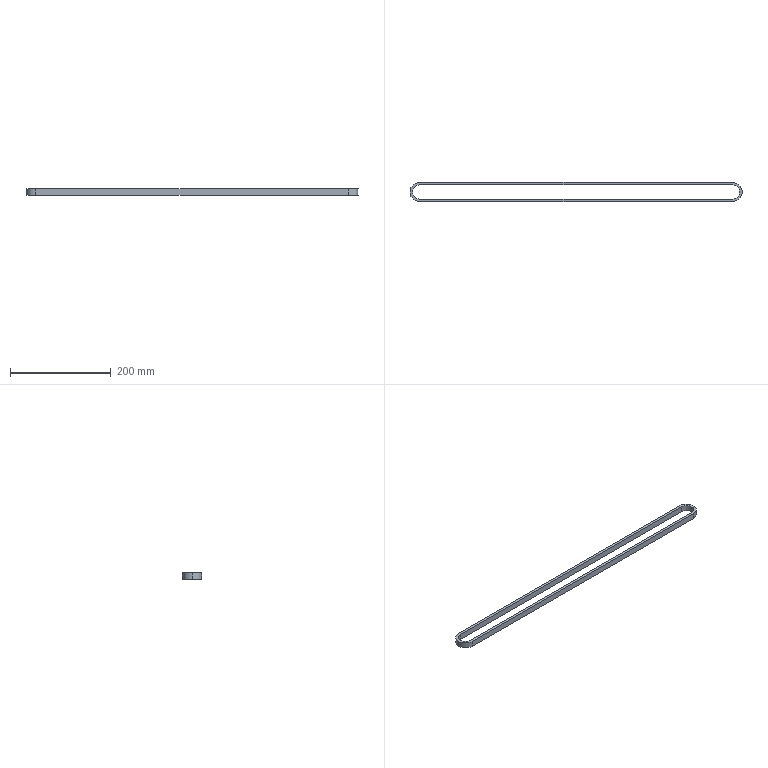Part | STEP file | 1/4in chain | 1 solid | 12 faces | box 658 x 38 x 12 mm | volume 80620 mm3 | cylinder 6 | plane 6 | commonest cylinder face diameters 28 x3 38 x3
STEP:
#1=CARTESIAN_POINT('',(0.,0.,0.));
#2=DIRECTION('',(0.,0.,1.));
#3=DIRECTION('',(1.,0.,0.));
#4=AXIS2_PLACEMENT_3D('',#1,#2,#3);
#5=CARTESIAN_POINT('',(-310.,14.,6.));
#6=VERTEX_POINT('',#5);
#7=CARTESIAN_POINT('',(-310.,14.,-6.));
#8=VERTEX_POINT('',#7);
#9=CARTESIAN_POINT('',(-310.,14.,6.));
#10=DIRECTION('',(0.,0.,-1.));
#11=VECTOR('',#10,1.);
#12=LINE('',#9,#11);
#13=CARTESIAN_POINT('',(-310.,0.,6.));
#14=DIRECTION('',(0.,0.,-1.));
#15=DIRECTION('',(-1.,0.,0.));
#16=AXIS2_PLACEMENT_3D('',#13,#14,#15);
#17=CYLINDRICAL_SURFACE('',#16,14.);
#18=CARTESIAN_POINT('',(1.571,0.));
#19=DIRECTION('',(0.,1.));
#20=VECTOR('',#19,1.);
#21=LINE('',#18,#20);
#22=(GEOMETRIC_REPRESENTATION_CONTEXT(2)PARAMETRIC_REPRESENTATION_CONTEXT()REPRESENTATION_CONTEXT('',''));
#23=DEFINITIONAL_REPRESENTATION('',(#21),#22);
#24=PCURVE('',#17,#23);
#25=CARTESIAN_POINT('',(-310.,14.,6.));
#26=DIRECTION('',(0.,-1.,0.));
#27=DIRECTION('',(1.,0.,0.));
#28=AXIS2_PLACEMENT_3D('',#25,#26,#27);
#29=PLANE('',#28);
#30=CARTESIAN_POINT('',(0.,0.));
#31=DIRECTION('',(0.,-1.));
#32=VECTOR('',#31,1.);
#33=LINE('',#30,#32);
#34=(GEOMETRIC_REPRESENTATION_CONTEXT(2)PARAMETRIC_REPRESENTATION_CONTEXT()REPRESENTATION_CONTEXT('',''));
#35=DEFINITIONAL_REPRESENTATION('',(#33),#34);
#36=PCURVE('',#29,#35);
#37=SURFACE_CURVE('',#12,(#24,#36),.PCURVE_S1.);
#38=EDGE_CURVE('',#6,#8,#37,.T.);
#39=ORIENTED_EDGE('',*,*,#38,.T.);
#40=CARTESIAN_POINT('',(-324.,0.,-6.));
#41=VERTEX_POINT('',#40);
#42=CARTESIAN_POINT('',(-310.,0.,-6.));
#43=DIRECTION('',(0.,0.,1.));
#44=DIRECTION('',(1.,0.,0.));
#45=AXIS2_PLACEMENT_3D('',#42,#43,#44);
#46=CIRCLE('',#45,14.);
#47=CARTESIAN_POINT('',(3.142,12.));
#48=DIRECTION('',(-1.,0.));
#49=VECTOR('',#48,1.);
#50=LINE('',#47,#49);
#51=(GEOMETRIC_REPRESENTATION_CONTEXT(2)PARAMETRIC_REPRESENTATION_CONTEXT()REPRESENTATION_CONTEXT('',''));
#52=DEFINITIONAL_REPRESENTATION('',(#50),#51);
#53=PCURVE('',#17,#52);
#54=CARTESIAN_POINT('',(-310.,0.,-6.));
#55=DIRECTION('',(0.,0.,1.));
#56=DIRECTION('',(1.,0.,0.));
#57=AXIS2_PLACEMENT_3D('',#54,#55,#56);
#58=PLANE('',#57);
#59=CARTESIAN_POINT('',(0.,0.));
#60=DIRECTION('',(1.,0.));
#61=AXIS2_PLACEMENT_2D('',#59,#60);
#62=CIRCLE('',#61,14.);
#63=(GEOMETRIC_REPRESENTATION_CONTEXT(2)PARAMETRIC_REPRESENTATION_CONTEXT()REPRESENTATION_CONTEXT('',''));
#64=DEFINITIONAL_REPRESENTATION('',(#62),#63);
#65=PCURVE('',#58,#64);
#66=SURFACE_CURVE('',#46,(#53,#65),.PCURVE_S1.);
#67=EDGE_CURVE('',#8,#41,#66,.T.);
#68=ORIENTED_EDGE('',*,*,#67,.T.);
#69=CARTESIAN_POINT('',(-324.,0.,6.));
#70=VERTEX_POINT('',#69);
#71=CARTESIAN_POINT('',(-324.,0.,6.));
#72=DIRECTION('',(0.,0.,-1.));
#73=VECTOR('',#72,1.);
#74=LINE('',#71,#73);
#75=CARTESIAN_POINT('',(0.,0.));
#76=DIRECTION('',(0.,1.));
#77=VECTOR('',#76,1.);
#78=LINE('',#75,#77);
#79=(GEOMETRIC_REPRESENTATION_CONTEXT(2)PARAMETRIC_REPRESENTATION_CONTEXT()REPRESENTATION_CONTEXT('',''));
#80=DEFINITIONAL_REPRESENTATION('',(#78),#79);
#81=PCURVE('',#17,#80);
#82=CARTESIAN_POINT('',(-310.,0.,6.));
#83=DIRECTION('',(0.,0.,-1.));
#84=DIRECTION('',(-1.,0.,0.));
#85=AXIS2_PLACEMENT_3D('',#82,#83,#84);
#86=CYLINDRICAL_SURFACE('',#85,14.);
#87=CARTESIAN_POINT('',(6.283,0.));
#88=DIRECTION('',(0.,1.));
#89=VECTOR('',#88,1.);
#90=LINE('',#87,#89);
#91=(GEOMETRIC_REPRESENTATION_CONTEXT(2)PARAMETRIC_REPRESENTATION_CONTEXT()REPRESENTATION_CONTEXT('',''));
#92=DEFINITIONAL_REPRESENTATION('',(#90),#91);
#93=PCURVE('',#86,#92);
#94=SURFACE_CURVE('',#74,(#81,#93),.PCURVE_S1.);
#95=EDGE_CURVE('',#70,#41,#94,.T.);
#96=ORIENTED_EDGE('',*,*,#95,.F.);
#97=CARTESIAN_POINT('',(-310.,0.,6.));
#98=DIRECTION('',(0.,0.,1.));
#99=DIRECTION('',(1.,0.,0.));
#100=AXIS2_PLACEMENT_3D('',#97,#98,#99);
#101=CIRCLE('',#100,14.);
#102=CARTESIAN_POINT('',(3.142,0.));
#103=DIRECTION('',(-1.,0.));
#104=VECTOR('',#103,1.);
#105=LINE('',#102,#104);
#106=(GEOMETRIC_REPRESENTATION_CONTEXT(2)PARAMETRIC_REPRESENTATION_CONTEXT()REPRESENTATION_CONTEXT('',''));
#107=DEFINITIONAL_REPRESENTATION('',(#105),#106);
#108=PCURVE('',#17,#107);
#109=CARTESIAN_POINT('',(-310.,0.,6.));
#110=DIRECTION('',(0.,0.,1.));
#111=DIRECTION('',(1.,0.,0.));
#112=AXIS2_PLACEMENT_3D('',#109,#110,#111);
#113=PLANE('',#112);
#114=CARTESIAN_POINT('',(0.,0.));
#115=DIRECTION('',(1.,0.));
#116=AXIS2_PLACEMENT_2D('',#114,#115);
#117=CIRCLE('',#116,14.);
#118=(GEOMETRIC_REPRESENTATION_CONTEXT(2)PARAMETRIC_REPRESENTATION_CONTEXT()REPRESENTATION_CONTEXT('',''));
#119=DEFINITIONAL_REPRESENTATION('',(#117),#118);
#120=PCURVE('',#113,#119);
#121=SURFACE_CURVE('',#101,(#108,#120),.PCURVE_S1.);
#122=EDGE_CURVE('',#6,#70,#121,.T.);
#123=ORIENTED_EDGE('',*,*,#122,.F.);
#124=EDGE_LOOP('',(#39,#68,#96,#123));
#125=FACE_BOUND('',#124,.F.);
#126=ADVANCED_FACE('',(#125),#17,.F.);
#127=CARTESIAN_POINT('',(-329.,0.,6.));
#128=VERTEX_POINT('',#127);
#129=CARTESIAN_POINT('',(-310.,-19.,6.));
#130=VERTEX_POINT('',#129);
#131=CARTESIAN_POINT('',(-310.,0.,6.));
#132=DIRECTION('',(0.,0.,1.));
#133=DIRECTION('',(1.,0.,0.));
#134=AXIS2_PLACEMENT_3D('',#131,#132,#133);
#135=CIRCLE('',#134,19.);
#136=CARTESIAN_POINT('',(-310.,0.,6.));
#137=DIRECTION('',(0.,0.,-1.));
#138=DIRECTION('',(-1.,0.,0.));
#139=AXIS2_PLACEMENT_3D('',#136,#137,#138);
#140=CYLINDRICAL_SURFACE('',#139,19.);
#141=CARTESIAN_POINT('',(9.425,0.));
#142=DIRECTION('',(-1.,0.));
#143=VECTOR('',#142,1.);
#144=LINE('',#141,#143);
#145=(GEOMETRIC_REPRESENTATION_CONTEXT(2)PARAMETRIC_REPRESENTATION_CONTEXT()REPRESENTATION_CONTEXT('',''));
#146=DEFINITIONAL_REPRESENTATION('',(#144),#145);
#147=PCURVE('',#140,#146);
#148=CARTESIAN_POINT('',(0.,0.));
#149=DIRECTION('',(1.,0.));
#150=AXIS2_PLACEMENT_2D('',#148,#149);
#151=CIRCLE('',#150,19.);
#152=(GEOMETRIC_REPRESENTATION_CONTEXT(2)PARAMETRIC_REPRESENTATION_CONTEXT()REPRESENTATION_CONTEXT('',''));
#153=DEFINITIONAL_REPRESENTATION('',(#151),#152);
#154=PCURVE('',#113,#153);
#155=SURFACE_CURVE('',#135,(#147,#154),.PCURVE_S1.);
#156=EDGE_CURVE('',#128,#130,#155,.T.);
#157=ORIENTED_EDGE('',*,*,#156,.F.);
#158=CARTESIAN_POINT('',(-329.,0.,-6.));
#159=VERTEX_POINT('',#158);
#160=CARTESIAN_POINT('',(-329.,0.,6.));
#161=DIRECTION('',(0.,0.,-1.));
#162=VECTOR('',#161,1.);
#163=LINE('',#160,#162);
#164=CARTESIAN_POINT('',(6.283,0.));
#165=DIRECTION('',(0.,1.));
#166=VECTOR('',#165,1.);
#167=LINE('',#164,#166);
#168=(GEOMETRIC_REPRESENTATION_CONTEXT(2)PARAMETRIC_REPRESENTATION_CONTEXT()REPRESENTATION_CONTEXT('',''));
#169=DEFINITIONAL_REPRESENTATION('',(#167),#168);
#170=PCURVE('',#140,#169);
#171=CARTESIAN_POINT('',(-310.,0.,6.));
#172=DIRECTION('',(0.,0.,-1.));
#173=DIRECTION('',(-1.,0.,0.));
#174=AXIS2_PLACEMENT_3D('',#171,#172,#173);
#175=CYLINDRICAL_SURFACE('',#174,19.);
#176=CARTESIAN_POINT('',(0.,0.));
#177=DIRECTION('',(0.,1.));
#178=VECTOR('',#177,1.);
#179=LINE('',#176,#178);
#180=(GEOMETRIC_REPRESENTATION_CONTEXT(2)PARAMETRIC_REPRESENTATION_CONTEXT()REPRESENTATION_CONTEXT('',''));
#181=DEFINITIONAL_REPRESENTATION('',(#179),#180);
#182=PCURVE('',#175,#181);
#183=SURFACE_CURVE('',#163,(#170,#182),.PCURVE_S1.);
#184=EDGE_CURVE('',#128,#159,#183,.T.);
#185=ORIENTED_EDGE('',*,*,#184,.T.);
#186=CARTESIAN_POINT('',(-310.,-19.,-6.));
#187=VERTEX_POINT('',#186);
#188=CARTESIAN_POINT('',(-310.,0.,-6.));
#189=DIRECTION('',(0.,0.,1.));
#190=DIRECTION('',(1.,0.,0.));
#191=AXIS2_PLACEMENT_3D('',#188,#189,#190);
#192=CIRCLE('',#191,19.);
#193=CARTESIAN_POINT('',(9.425,12.));
#194=DIRECTION('',(-1.,0.));
#195=VECTOR('',#194,1.);
#196=LINE('',#193,#195);
#197=(GEOMETRIC_REPRESENTATION_CONTEXT(2)PARAMETRIC_REPRESENTATION_CONTEXT()REPRESENTATION_CONTEXT('',''));
#198=DEFINITIONAL_REPRESENTATION('',(#196),#197);
#199=PCURVE('',#140,#198);
#200=CARTESIAN_POINT('',(0.,0.));
#201=DIRECTION('',(1.,0.));
#202=AXIS2_PLACEMENT_2D('',#200,#201);
#203=CIRCLE('',#202,19.);
#204=(GEOMETRIC_REPRESENTATION_CONTEXT(2)PARAMETRIC_REPRESENTATION_CONTEXT()REPRESENTATION_CONTEXT('',''));
#205=DEFINITIONAL_REPRESENTATION('',(#203),#204);
#206=PCURVE('',#58,#205);
#207=SURFACE_CURVE('',#192,(#199,#206),.PCURVE_S1.);
#208=EDGE_CURVE('',#159,#187,#207,.T.);
#209=ORIENTED_EDGE('',*,*,#208,.T.);
#210=CARTESIAN_POINT('',(-310.,-19.,6.));
#211=DIRECTION('',(0.,0.,-1.));
#212=VECTOR('',#211,1.);
#213=LINE('',#210,#212);
#214=CARTESIAN_POINT('',(4.712,0.));
#215=DIRECTION('',(0.,1.));
#216=VECTOR('',#215,1.);
#217=LINE('',#214,#216);
#218=(GEOMETRIC_REPRESENTATION_CONTEXT(2)PARAMETRIC_REPRESENTATION_CONTEXT()REPRESENTATION_CONTEXT('',''));
#219=DEFINITIONAL_REPRESENTATION('',(#217),#218);
#220=PCURVE('',#140,#219);
#221=CARTESIAN_POINT('',(-310.,-19.,6.));
#222=DIRECTION('',(0.,1.,0.));
#223=DIRECTION('',(-1.,0.,0.));
#224=AXIS2_PLACEMENT_3D('',#221,#222,#223);
#225=PLANE('',#224);
#226=CARTESIAN_POINT('',(0.,0.));
#227=DIRECTION('',(0.,-1.));
#228=VECTOR('',#227,1.);
#229=LINE('',#226,#228);
#230=(GEOMETRIC_REPRESENTATION_CONTEXT(2)PARAMETRIC_REPRESENTATION_CONTEXT()REPRESENTATION_CONTEXT('',''));
#231=DEFINITIONAL_REPRESENTATION('',(#229),#230);
#232=PCURVE('',#225,#231);
#233=SURFACE_CURVE('',#213,(#220,#232),.PCURVE_S1.);
#234=EDGE_CURVE('',#130,#187,#233,.T.);
#235=ORIENTED_EDGE('',*,*,#234,.F.);
#236=EDGE_LOOP('',(#157,#185,#209,#235));
#237=FACE_BOUND('',#236,.T.);
#238=ADVANCED_FACE('',(#237),#140,.T.);
#239=CARTESIAN_POINT('',(-310.,19.,6.));
#240=VERTEX_POINT('',#239);
#241=CARTESIAN_POINT('',(-310.,0.,6.));
#242=DIRECTION('',(0.,0.,1.));
#243=DIRECTION('',(1.,0.,0.));
#244=AXIS2_PLACEMENT_3D('',#241,#242,#243);
#245=CIRCLE('',#244,19.);
#246=CARTESIAN_POINT('',(0.,0.));
#247=DIRECTION('',(1.,0.));
#248=AXIS2_PLACEMENT_2D('',#246,#247);
#249=CIRCLE('',#248,19.);
#250=(GEOMETRIC_REPRESENTATION_CONTEXT(2)PARAMETRIC_REPRESENTATION_CONTEXT()REPRESENTATION_CONTEXT('',''));
#251=DEFINITIONAL_REPRESENTATION('',(#249),#250);
#252=PCURVE('',#113,#251);
#253=CARTESIAN_POINT('',(3.142,0.));
#254=DIRECTION('',(-1.,0.));
#255=VECTOR('',#254,1.);
#256=LINE('',#253,#255);
#257=(GEOMETRIC_REPRESENTATION_CONTEXT(2)PARAMETRIC_REPRESENTATION_CONTEXT()REPRESENTATION_CONTEXT('',''));
#258=DEFINITIONAL_REPRESENTATION('',(#256),#257);
#259=PCURVE('',#175,#258);
#260=SURFACE_CURVE('',#245,(#252,#259),.PCURVE_S1.);
#261=EDGE_CURVE('',#240,#128,#260,.T.);
#262=ORIENTED_EDGE('',*,*,#261,.T.);
#263=ORIENTED_EDGE('',*,*,#156,.T.);
#264=CARTESIAN_POINT('',(310.,-19.,6.));
#265=VERTEX_POINT('',#264);
#266=CARTESIAN_POINT('',(-310.,-19.,6.));
#267=DIRECTION('',(1.,0.,0.));
#268=VECTOR('',#267,1.);
#269=LINE('',#266,#268);
#270=CARTESIAN_POINT('',(0.,-19.));
#271=DIRECTION('',(1.,0.));
#272=VECTOR('',#271,1.);
#273=LINE('',#270,#272);
#274=(GEOMETRIC_REPRESENTATION_CONTEXT(2)PARAMETRIC_REPRESENTATION_CONTEXT()REPRESENTATION_CONTEXT('',''));
#275=DEFINITIONAL_REPRESENTATION('',(#273),#274);
#276=PCURVE('',#113,#275);
#277=CARTESIAN_POINT('',(0.,0.));
#278=DIRECTION('',(-1.,0.));
#279=VECTOR('',#278,1.);
#280=LINE('',#277,#279);
#281=(GEOMETRIC_REPRESENTATION_CONTEXT(2)PARAMETRIC_REPRESENTATION_CONTEXT()REPRESENTATION_CONTEXT('',''));
#282=DEFINITIONAL_REPRESENTATION('',(#280),#281);
#283=PCURVE('',#225,#282);
#284=SURFACE_CURVE('',#269,(#276,#283),.PCURVE_S1.);
#285=EDGE_CURVE('',#130,#265,#284,.T.);
#286=ORIENTED_EDGE('',*,*,#285,.T.);
#287=CARTESIAN_POINT('',(310.,19.,6.));
#288=VERTEX_POINT('',#287);
#289=CARTESIAN_POINT('',(310.,0.,6.));
#290=DIRECTION('',(0.,0.,1.));
#291=DIRECTION('',(-1.,0.,0.));
#292=AXIS2_PLACEMENT_3D('',#289,#290,#291);
#293=CIRCLE('',#292,19.);
#294=CARTESIAN_POINT('',(620.,0.));
#295=DIRECTION('',(-1.,0.));
#296=AXIS2_PLACEMENT_2D('',#294,#295);
#297=CIRCLE('',#296,19.);
#298=(GEOMETRIC_REPRESENTATION_CONTEXT(2)PARAMETRIC_REPRESENTATION_CONTEXT()REPRESENTATION_CONTEXT('',''));
#299=DEFINITIONAL_REPRESENTATION('',(#297),#298);
#300=PCURVE('',#113,#299);
#301=CARTESIAN_POINT('',(310.,0.,6.));
#302=DIRECTION('',(0.,0.,-1.));
#303=DIRECTION('',(-1.,0.,0.));
#304=AXIS2_PLACEMENT_3D('',#301,#302,#303);
#305=CYLINDRICAL_SURFACE('',#304,19.);
#306=CARTESIAN_POINT('',(6.283,0.));
#307=DIRECTION('',(-1.,0.));
#308=VECTOR('',#307,1.);
#309=LINE('',#306,#308);
#310=(GEOMETRIC_REPRESENTATION_CONTEXT(2)PARAMETRIC_REPRESENTATION_CONTEXT()REPRESENTATION_CONTEXT('',''));
#311=DEFINITIONAL_REPRESENTATION('',(#309),#310);
#312=PCURVE('',#305,#311);
#313=SURFACE_CURVE('',#293,(#300,#312),.PCURVE_S1.);
#314=EDGE_CURVE('',#265,#288,#313,.T.);
#315=ORIENTED_EDGE('',*,*,#314,.T.);
#316=CARTESIAN_POINT('',(-310.,19.,6.));
#317=DIRECTION('',(-1.,0.,0.));
#318=VECTOR('',#317,1.);
#319=LINE('',#316,#318);
#320=CARTESIAN_POINT('',(0.,19.));
#321=DIRECTION('',(-1.,0.));
#322=VECTOR('',#321,1.);
#323=LINE('',#320,#322);
#324=(GEOMETRIC_REPRESENTATION_CONTEXT(2)PARAMETRIC_REPRESENTATION_CONTEXT()REPRESENTATION_CONTEXT('',''));
#325=DEFINITIONAL_REPRESENTATION('',(#323),#324);
#326=PCURVE('',#113,#325);
#327=CARTESIAN_POINT('',(-310.,19.,6.));
#328=DIRECTION('',(0.,-1.,0.));
#329=DIRECTION('',(1.,0.,0.));
#330=AXIS2_PLACEMENT_3D('',#327,#328,#329);
#331=PLANE('',#330);
#332=CARTESIAN_POINT('',(0.,0.));
#333=DIRECTION('',(-1.,0.));
#334=VECTOR('',#333,1.);
#335=LINE('',#332,#334);
#336=(GEOMETRIC_REPRESENTATION_CONTEXT(2)PARAMETRIC_REPRESENTATION_CONTEXT()REPRESENTATION_CONTEXT('',''));
#337=DEFINITIONAL_REPRESENTATION('',(#335),#336);
#338=PCURVE('',#331,#337);
#339=SURFACE_CURVE('',#319,(#326,#338),.PCURVE_S1.);
#340=EDGE_CURVE('',#288,#240,#339,.T.);
#341=ORIENTED_EDGE('',*,*,#340,.T.);
#342=EDGE_LOOP('',(#262,#263,#286,#315,#341));
#343=FACE_BOUND('',#342,.T.);
#344=CARTESIAN_POINT('',(-310.,-14.,6.));
#345=VERTEX_POINT('',#344);
#346=CARTESIAN_POINT('',(310.,-14.,6.));
#347=VERTEX_POINT('',#346);
#348=CARTESIAN_POINT('',(-310.,-14.,6.));
#349=DIRECTION('',(1.,0.,0.));
#350=VECTOR('',#349,1.);
#351=LINE('',#348,#350);
#352=CARTESIAN_POINT('',(0.,-14.));
#353=DIRECTION('',(1.,0.));
#354=VECTOR('',#353,1.);
#355=LINE('',#352,#354);
#356=(GEOMETRIC_REPRESENTATION_CONTEXT(2)PARAMETRIC_REPRESENTATION_CONTEXT()REPRESENTATION_CONTEXT('',''));
#357=DEFINITIONAL_REPRESENTATION('',(#355),#356);
#358=PCURVE('',#113,#357);
#359=CARTESIAN_POINT('',(-310.,-14.,6.));
#360=DIRECTION('',(0.,1.,0.));
#361=DIRECTION('',(-1.,0.,0.));
#362=AXIS2_PLACEMENT_3D('',#359,#360,#361);
#363=PLANE('',#362);
#364=CARTESIAN_POINT('',(0.,0.));
#365=DIRECTION('',(-1.,0.));
#366=VECTOR('',#365,1.);
#367=LINE('',#364,#366);
#368=(GEOMETRIC_REPRESENTATION_CONTEXT(2)PARAMETRIC_REPRESENTATION_CONTEXT()REPRESENTATION_CONTEXT('',''));
#369=DEFINITIONAL_REPRESENTATION('',(#367),#368);
#370=PCURVE('',#363,#369);
#371=SURFACE_CURVE('',#351,(#358,#370),.PCURVE_S1.);
#372=EDGE_CURVE('',#345,#347,#371,.T.);
#373=ORIENTED_EDGE('',*,*,#372,.F.);
#374=CARTESIAN_POINT('',(-310.,0.,6.));
#375=DIRECTION('',(0.,0.,1.));
#376=DIRECTION('',(1.,0.,0.));
#377=AXIS2_PLACEMENT_3D('',#374,#375,#376);
#378=CIRCLE('',#377,14.);
#379=CARTESIAN_POINT('',(0.,0.));
#380=DIRECTION('',(1.,0.));
#381=AXIS2_PLACEMENT_2D('',#379,#380);
#382=CIRCLE('',#381,14.);
#383=(GEOMETRIC_REPRESENTATION_CONTEXT(2)PARAMETRIC_REPRESENTATION_CONTEXT()REPRESENTATION_CONTEXT('',''));
#384=DEFINITIONAL_REPRESENTATION('',(#382),#383);
#385=PCURVE('',#113,#384);
#386=CARTESIAN_POINT('',(9.425,0.));
#387=DIRECTION('',(-1.,0.));
#388=VECTOR('',#387,1.);
#389=LINE('',#386,#388);
#390=(GEOMETRIC_REPRESENTATION_CONTEXT(2)PARAMETRIC_REPRESENTATION_CONTEXT()REPRESENTATION_CONTEXT('',''));
#391=DEFINITIONAL_REPRESENTATION('',(#389),#390);
#392=PCURVE('',#86,#391);
#393=SURFACE_CURVE('',#378,(#385,#392),.PCURVE_S1.);
#394=EDGE_CURVE('',#70,#345,#393,.T.);
#395=ORIENTED_EDGE('',*,*,#394,.F.);
#396=ORIENTED_EDGE('',*,*,#122,.F.);
#397=CARTESIAN_POINT('',(310.,14.,6.));
#398=VERTEX_POINT('',#397);
#399=CARTESIAN_POINT('',(-310.,14.,6.));
#400=DIRECTION('',(-1.,0.,0.));
#401=VECTOR('',#400,1.);
#402=LINE('',#399,#401);
#403=CARTESIAN_POINT('',(0.,14.));
#404=DIRECTION('',(-1.,0.));
#405=VECTOR('',#404,1.);
#406=LINE('',#403,#405);
#407=(GEOMETRIC_REPRESENTATION_CONTEXT(2)PARAMETRIC_REPRESENTATION_CONTEXT()REPRESENTATION_CONTEXT('',''));
#408=DEFINITIONAL_REPRESENTATION('',(#406),#407);
#409=PCURVE('',#113,#408);
#410=CARTESIAN_POINT('',(0.,0.));
#411=DIRECTION('',(-1.,0.));
#412=VECTOR('',#411,1.);
#413=LINE('',#410,#412);
#414=(GEOMETRIC_REPRESENTATION_CONTEXT(2)PARAMETRIC_REPRESENTATION_CONTEXT()REPRESENTATION_CONTEXT('',''));
#415=DEFINITIONAL_REPRESENTATION('',(#413),#414);
#416=PCURVE('',#29,#415);
#417=SURFACE_CURVE('',#402,(#409,#416),.PCURVE_S1.);
#418=EDGE_CURVE('',#398,#6,#417,.T.);
#419=ORIENTED_EDGE('',*,*,#418,.F.);
#420=CARTESIAN_POINT('',(310.,0.,6.));
#421=DIRECTION('',(0.,0.,1.));
#422=DIRECTION('',(1.,0.,0.));
#423=AXIS2_PLACEMENT_3D('',#420,#421,#422);
#424=CIRCLE('',#423,14.);
#425=CARTESIAN_POINT('',(620.,0.));
#426=DIRECTION('',(1.,0.));
#427=AXIS2_PLACEMENT_2D('',#425,#426);
#428=CIRCLE('',#427,14.);
#429=(GEOMETRIC_REPRESENTATION_CONTEXT(2)PARAMETRIC_REPRESENTATION_CONTEXT()REPRESENTATION_CONTEXT('',''));
#430=DEFINITIONAL_REPRESENTATION('',(#428),#429);
#431=PCURVE('',#113,#430);
#432=CARTESIAN_POINT('',(310.,0.,6.));
#433=DIRECTION('',(0.,0.,-1.));
#434=DIRECTION('',(-1.,0.,0.));
#435=AXIS2_PLACEMENT_3D('',#432,#433,#434);
#436=CYLINDRICAL_SURFACE('',#435,14.);
#437=CARTESIAN_POINT('',(9.425,0.));
#438=DIRECTION('',(-1.,0.));
#439=VECTOR('',#438,1.);
#440=LINE('',#437,#439);
#441=(GEOMETRIC_REPRESENTATION_CONTEXT(2)PARAMETRIC_REPRESENTATION_CONTEXT()REPRESENTATION_CONTEXT('',''));
#442=DEFINITIONAL_REPRESENTATION('',(#440),#441);
#443=PCURVE('',#436,#442);
#444=SURFACE_CURVE('',#424,(#431,#443),.PCURVE_S1.);
#445=EDGE_CURVE('',#347,#398,#444,.T.);
#446=ORIENTED_EDGE('',*,*,#445,.F.);
#447=EDGE_LOOP('',(#373,#395,#396,#419,#446));
#448=FACE_BOUND('',#447,.T.);
#449=ADVANCED_FACE('',(#343,#448),#113,.T.);
#450=CARTESIAN_POINT('',(-310.,19.,-6.));
#451=VERTEX_POINT('',#450);
#452=CARTESIAN_POINT('',(-310.,0.,-6.));
#453=DIRECTION('',(0.,0.,1.));
#454=DIRECTION('',(1.,0.,0.));
#455=AXIS2_PLACEMENT_3D('',#452,#453,#454);
#456=CIRCLE('',#455,19.);
#457=CARTESIAN_POINT('',(0.,0.));
#458=DIRECTION('',(1.,0.));
#459=AXIS2_PLACEMENT_2D('',#457,#458);
#460=CIRCLE('',#459,19.);
#461=(GEOMETRIC_REPRESENTATION_CONTEXT(2)PARAMETRIC_REPRESENTATION_CONTEXT()REPRESENTATION_CONTEXT('',''));
#462=DEFINITIONAL_REPRESENTATION('',(#460),#461);
#463=PCURVE('',#58,#462);
#464=CARTESIAN_POINT('',(3.142,12.));
#465=DIRECTION('',(-1.,0.));
#466=VECTOR('',#465,1.);
#467=LINE('',#464,#466);
#468=(GEOMETRIC_REPRESENTATION_CONTEXT(2)PARAMETRIC_REPRESENTATION_CONTEXT()REPRESENTATION_CONTEXT('',''));
#469=DEFINITIONAL_REPRESENTATION('',(#467),#468);
#470=PCURVE('',#175,#469);
#471=SURFACE_CURVE('',#456,(#463,#470),.PCURVE_S1.);
#472=EDGE_CURVE('',#451,#159,#471,.T.);
#473=ORIENTED_EDGE('',*,*,#472,.F.);
#474=CARTESIAN_POINT('',(310.,19.,-6.));
#475=VERTEX_POINT('',#474);
#476=CARTESIAN_POINT('',(-310.,19.,-6.));
#477=DIRECTION('',(-1.,0.,0.));
#478=VECTOR('',#477,1.);
#479=LINE('',#476,#478);
#480=CARTESIAN_POINT('',(0.,19.));
#481=DIRECTION('',(-1.,0.));
#482=VECTOR('',#481,1.);
#483=LINE('',#480,#482);
#484=(GEOMETRIC_REPRESENTATION_CONTEXT(2)PARAMETRIC_REPRESENTATION_CONTEXT()REPRESENTATION_CONTEXT('',''));
#485=DEFINITIONAL_REPRESENTATION('',(#483),#484);
#486=PCURVE('',#58,#485);
#487=CARTESIAN_POINT('',(0.,-12.));
#488=DIRECTION('',(-1.,0.));
#489=VECTOR('',#488,1.);
#490=LINE('',#487,#489);
#491=(GEOMETRIC_REPRESENTATION_CONTEXT(2)PARAMETRIC_REPRESENTATION_CONTEXT()REPRESENTATION_CONTEXT('',''));
#492=DEFINITIONAL_REPRESENTATION('',(#490),#491);
#493=PCURVE('',#331,#492);
#494=SURFACE_CURVE('',#479,(#486,#493),.PCURVE_S1.);
#495=EDGE_CURVE('',#475,#451,#494,.T.);
#496=ORIENTED_EDGE('',*,*,#495,.F.);
#497=CARTESIAN_POINT('',(310.,-19.,-6.));
#498=VERTEX_POINT('',#497);
#499=CARTESIAN_POINT('',(310.,0.,-6.));
#500=DIRECTION('',(0.,0.,1.));
#501=DIRECTION('',(-1.,0.,0.));
#502=AXIS2_PLACEMENT_3D('',#499,#500,#501);
#503=CIRCLE('',#502,19.);
#504=CARTESIAN_POINT('',(620.,0.));
#505=DIRECTION('',(-1.,0.));
#506=AXIS2_PLACEMENT_2D('',#504,#505);
#507=CIRCLE('',#506,19.);
#508=(GEOMETRIC_REPRESENTATION_CONTEXT(2)PARAMETRIC_REPRESENTATION_CONTEXT()REPRESENTATION_CONTEXT('',''));
#509=DEFINITIONAL_REPRESENTATION('',(#507),#508);
#510=PCURVE('',#58,#509);
#511=CARTESIAN_POINT('',(6.283,12.));
#512=DIRECTION('',(-1.,0.));
#513=VECTOR('',#512,1.);
#514=LINE('',#511,#513);
#515=(GEOMETRIC_REPRESENTATION_CONTEXT(2)PARAMETRIC_REPRESENTATION_CONTEXT()REPRESENTATION_CONTEXT('',''));
#516=DEFINITIONAL_REPRESENTATION('',(#514),#515);
#517=PCURVE('',#305,#516);
#518=SURFACE_CURVE('',#503,(#510,#517),.PCURVE_S1.);
#519=EDGE_CURVE('',#498,#475,#518,.T.);
#520=ORIENTED_EDGE('',*,*,#519,.F.);
#521=CARTESIAN_POINT('',(-310.,-19.,-6.));
#522=DIRECTION('',(1.,0.,0.));
#523=VECTOR('',#522,1.);
#524=LINE('',#521,#523);
#525=CARTESIAN_POINT('',(0.,-19.));
#526=DIRECTION('',(1.,0.));
#527=VECTOR('',#526,1.);
#528=LINE('',#525,#527);
#529=(GEOMETRIC_REPRESENTATION_CONTEXT(2)PARAMETRIC_REPRESENTATION_CONTEXT()REPRESENTATION_CONTEXT('',''));
#530=DEFINITIONAL_REPRESENTATION('',(#528),#529);
#531=PCURVE('',#58,#530);
#532=CARTESIAN_POINT('',(0.,-12.));
#533=DIRECTION('',(-1.,0.));
#534=VECTOR('',#533,1.);
#535=LINE('',#532,#534);
#536=(GEOMETRIC_REPRESENTATION_CONTEXT(2)PARAMETRIC_REPRESENTATION_CONTEXT()REPRESENTATION_CONTEXT('',''));
#537=DEFINITIONAL_REPRESENTATION('',(#535),#536);
#538=PCURVE('',#225,#537);
#539=SURFACE_CURVE('',#524,(#531,#538),.PCURVE_S1.);
#540=EDGE_CURVE('',#187,#498,#539,.T.);
#541=ORIENTED_EDGE('',*,*,#540,.F.);
#542=ORIENTED_EDGE('',*,*,#208,.F.);
#543=EDGE_LOOP('',(#473,#496,#520,#541,#542));
#544=FACE_BOUND('',#543,.T.);
#545=ORIENTED_EDGE('',*,*,#67,.T.);
#546=CARTESIAN_POINT('',(-310.,-14.,-6.));
#547=VERTEX_POINT('',#546);
#548=CARTESIAN_POINT('',(-310.,0.,-6.));
#549=DIRECTION('',(0.,0.,1.));
#550=DIRECTION('',(1.,0.,0.));
#551=AXIS2_PLACEMENT_3D('',#548,#549,#550);
#552=CIRCLE('',#551,14.);
#553=CARTESIAN_POINT('',(0.,0.));
#554=DIRECTION('',(1.,0.));
#555=AXIS2_PLACEMENT_2D('',#553,#554);
#556=CIRCLE('',#555,14.);
#557=(GEOMETRIC_REPRESENTATION_CONTEXT(2)PARAMETRIC_REPRESENTATION_CONTEXT()REPRESENTATION_CONTEXT('',''));
#558=DEFINITIONAL_REPRESENTATION('',(#556),#557);
#559=PCURVE('',#58,#558);
#560=CARTESIAN_POINT('',(9.425,12.));
#561=DIRECTION('',(-1.,0.));
#562=VECTOR('',#561,1.);
#563=LINE('',#560,#562);
#564=(GEOMETRIC_REPRESENTATION_CONTEXT(2)PARAMETRIC_REPRESENTATION_CONTEXT()REPRESENTATION_CONTEXT('',''));
#565=DEFINITIONAL_REPRESENTATION('',(#563),#564);
#566=PCURVE('',#86,#565);
#567=SURFACE_CURVE('',#552,(#559,#566),.PCURVE_S1.);
#568=EDGE_CURVE('',#41,#547,#567,.T.);
#569=ORIENTED_EDGE('',*,*,#568,.T.);
#570=CARTESIAN_POINT('',(310.,-14.,-6.));
#571=VERTEX_POINT('',#570);
#572=CARTESIAN_POINT('',(-310.,-14.,-6.));
#573=DIRECTION('',(1.,0.,0.));
#574=VECTOR('',#573,1.);
#575=LINE('',#572,#574);
#576=CARTESIAN_POINT('',(0.,-14.));
#577=DIRECTION('',(1.,0.));
#578=VECTOR('',#577,1.);
#579=LINE('',#576,#578);
#580=(GEOMETRIC_REPRESENTATION_CONTEXT(2)PARAMETRIC_REPRESENTATION_CONTEXT()REPRESENTATION_CONTEXT('',''));
#581=DEFINITIONAL_REPRESENTATION('',(#579),#580);
#582=PCURVE('',#58,#581);
#583=CARTESIAN_POINT('',(0.,-12.));
#584=DIRECTION('',(-1.,0.));
#585=VECTOR('',#584,1.);
#586=LINE('',#583,#585);
#587=(GEOMETRIC_REPRESENTATION_CONTEXT(2)PARAMETRIC_REPRESENTATION_CONTEXT()REPRESENTATION_CONTEXT('',''));
#588=DEFINITIONAL_REPRESENTATION('',(#586),#587);
#589=PCURVE('',#363,#588);
#590=SURFACE_CURVE('',#575,(#582,#589),.PCURVE_S1.);
#591=EDGE_CURVE('',#547,#571,#590,.T.);
#592=ORIENTED_EDGE('',*,*,#591,.T.);
#593=CARTESIAN_POINT('',(310.,14.,-6.));
#594=VERTEX_POINT('',#593);
#595=CARTESIAN_POINT('',(310.,0.,-6.));
#596=DIRECTION('',(0.,0.,1.));
#597=DIRECTION('',(1.,0.,0.));
#598=AXIS2_PLACEMENT_3D('',#595,#596,#597);
#599=CIRCLE('',#598,14.);
#600=CARTESIAN_POINT('',(620.,0.));
#601=DIRECTION('',(1.,0.));
#602=AXIS2_PLACEMENT_2D('',#600,#601);
#603=CIRCLE('',#602,14.);
#604=(GEOMETRIC_REPRESENTATION_CONTEXT(2)PARAMETRIC_REPRESENTATION_CONTEXT()REPRESENTATION_CONTEXT('',''));
#605=DEFINITIONAL_REPRESENTATION('',(#603),#604);
#606=PCURVE('',#58,#605);
#607=CARTESIAN_POINT('',(9.425,12.));
#608=DIRECTION('',(-1.,0.));
#609=VECTOR('',#608,1.);
#610=LINE('',#607,#609);
#611=(GEOMETRIC_REPRESENTATION_CONTEXT(2)PARAMETRIC_REPRESENTATION_CONTEXT()REPRESENTATION_CONTEXT('',''));
#612=DEFINITIONAL_REPRESENTATION('',(#610),#611);
#613=PCURVE('',#436,#612);
#614=SURFACE_CURVE('',#599,(#606,#613),.PCURVE_S1.);
#615=EDGE_CURVE('',#571,#594,#614,.T.);
#616=ORIENTED_EDGE('',*,*,#615,.T.);
#617=CARTESIAN_POINT('',(-310.,14.,-6.));
#618=DIRECTION('',(-1.,0.,0.));
#619=VECTOR('',#618,1.);
#620=LINE('',#617,#619);
#621=CARTESIAN_POINT('',(0.,14.));
#622=DIRECTION('',(-1.,0.));
#623=VECTOR('',#622,1.);
#624=LINE('',#621,#623);
#625=(GEOMETRIC_REPRESENTATION_CONTEXT(2)PARAMETRIC_REPRESENTATION_CONTEXT()REPRESENTATION_CONTEXT('',''));
#626=DEFINITIONAL_REPRESENTATION('',(#624),#625);
#627=PCURVE('',#58,#626);
#628=CARTESIAN_POINT('',(0.,-12.));
#629=DIRECTION('',(-1.,0.));
#630=VECTOR('',#629,1.);
#631=LINE('',#628,#630);
#632=(GEOMETRIC_REPRESENTATION_CONTEXT(2)PARAMETRIC_REPRESENTATION_CONTEXT()REPRESENTATION_CONTEXT('',''));
#633=DEFINITIONAL_REPRESENTATION('',(#631),#632);
#634=PCURVE('',#29,#633);
#635=SURFACE_CURVE('',#620,(#627,#634),.PCURVE_S1.);
#636=EDGE_CURVE('',#594,#8,#635,.T.);
#637=ORIENTED_EDGE('',*,*,#636,.T.);
#638=EDGE_LOOP('',(#545,#569,#592,#616,#637));
#639=FACE_BOUND('',#638,.T.);
#640=ADVANCED_FACE('',(#544,#639),#58,.F.);
#641=ORIENTED_EDGE('',*,*,#184,.F.);
#642=ORIENTED_EDGE('',*,*,#261,.F.);
#643=CARTESIAN_POINT('',(-310.,19.,6.));
#644=DIRECTION('',(0.,0.,-1.));
#645=VECTOR('',#644,1.);
#646=LINE('',#643,#645);
#647=CARTESIAN_POINT('',(1.571,0.));
#648=DIRECTION('',(0.,1.));
#649=VECTOR('',#648,1.);
#650=LINE('',#647,#649);
#651=(GEOMETRIC_REPRESENTATION_CONTEXT(2)PARAMETRIC_REPRESENTATION_CONTEXT()REPRESENTATION_CONTEXT('',''));
#652=DEFINITIONAL_REPRESENTATION('',(#650),#651);
#653=PCURVE('',#175,#652);
#654=CARTESIAN_POINT('',(0.,0.));
#655=DIRECTION('',(0.,-1.));
#656=VECTOR('',#655,1.);
#657=LINE('',#654,#656);
#658=(GEOMETRIC_REPRESENTATION_CONTEXT(2)PARAMETRIC_REPRESENTATION_CONTEXT()REPRESENTATION_CONTEXT('',''));
#659=DEFINITIONAL_REPRESENTATION('',(#657),#658);
#660=PCURVE('',#331,#659);
#661=SURFACE_CURVE('',#646,(#653,#660),.PCURVE_S1.);
#662=EDGE_CURVE('',#240,#451,#661,.T.);
#663=ORIENTED_EDGE('',*,*,#662,.T.);
#664=ORIENTED_EDGE('',*,*,#472,.T.);
#665=EDGE_LOOP('',(#641,#642,#663,#664));
#666=FACE_BOUND('',#665,.T.);
#667=ADVANCED_FACE('',(#666),#175,.T.);
#668=ORIENTED_EDGE('',*,*,#540,.T.);
#669=CARTESIAN_POINT('',(310.,-19.,6.));
#670=DIRECTION('',(0.,0.,-1.));
#671=VECTOR('',#670,1.);
#672=LINE('',#669,#671);
#673=CARTESIAN_POINT('',(-620.,0.));
#674=DIRECTION('',(0.,-1.));
#675=VECTOR('',#674,1.);
#676=LINE('',#673,#675);
#677=(GEOMETRIC_REPRESENTATION_CONTEXT(2)PARAMETRIC_REPRESENTATION_CONTEXT()REPRESENTATION_CONTEXT('',''));
#678=DEFINITIONAL_REPRESENTATION('',(#676),#677);
#679=PCURVE('',#225,#678);
#680=CARTESIAN_POINT('',(4.712,0.));
#681=DIRECTION('',(0.,1.));
#682=VECTOR('',#681,1.);
#683=LINE('',#680,#682);
#684=(GEOMETRIC_REPRESENTATION_CONTEXT(2)PARAMETRIC_REPRESENTATION_CONTEXT()REPRESENTATION_CONTEXT('',''));
#685=DEFINITIONAL_REPRESENTATION('',(#683),#684);
#686=PCURVE('',#305,#685);
#687=SURFACE_CURVE('',#672,(#679,#686),.PCURVE_S1.);
#688=EDGE_CURVE('',#265,#498,#687,.T.);
#689=ORIENTED_EDGE('',*,*,#688,.F.);
#690=ORIENTED_EDGE('',*,*,#285,.F.);
#691=ORIENTED_EDGE('',*,*,#234,.T.);
#692=EDGE_LOOP('',(#668,#689,#690,#691));
#693=FACE_BOUND('',#692,.T.);
#694=ADVANCED_FACE('',(#693),#225,.F.);
#695=ORIENTED_EDGE('',*,*,#519,.T.);
#696=CARTESIAN_POINT('',(310.,19.,6.));
#697=DIRECTION('',(0.,0.,-1.));
#698=VECTOR('',#697,1.);
#699=LINE('',#696,#698);
#700=CARTESIAN_POINT('',(1.571,0.));
#701=DIRECTION('',(0.,1.));
#702=VECTOR('',#701,1.);
#703=LINE('',#700,#702);
#704=(GEOMETRIC_REPRESENTATION_CONTEXT(2)PARAMETRIC_REPRESENTATION_CONTEXT()REPRESENTATION_CONTEXT('',''));
#705=DEFINITIONAL_REPRESENTATION('',(#703),#704);
#706=PCURVE('',#305,#705);
#707=CARTESIAN_POINT('',(620.,0.));
#708=DIRECTION('',(0.,-1.));
#709=VECTOR('',#708,1.);
#710=LINE('',#707,#709);
#711=(GEOMETRIC_REPRESENTATION_CONTEXT(2)PARAMETRIC_REPRESENTATION_CONTEXT()REPRESENTATION_CONTEXT('',''));
#712=DEFINITIONAL_REPRESENTATION('',(#710),#711);
#713=PCURVE('',#331,#712);
#714=SURFACE_CURVE('',#699,(#706,#713),.PCURVE_S1.);
#715=EDGE_CURVE('',#288,#475,#714,.T.);
#716=ORIENTED_EDGE('',*,*,#715,.F.);
#717=ORIENTED_EDGE('',*,*,#314,.F.);
#718=ORIENTED_EDGE('',*,*,#688,.T.);
#719=EDGE_LOOP('',(#695,#716,#717,#718));
#720=FACE_BOUND('',#719,.T.);
#721=ADVANCED_FACE('',(#720),#305,.T.);
#722=ORIENTED_EDGE('',*,*,#495,.T.);
#723=ORIENTED_EDGE('',*,*,#662,.F.);
#724=ORIENTED_EDGE('',*,*,#340,.F.);
#725=ORIENTED_EDGE('',*,*,#715,.T.);
#726=EDGE_LOOP('',(#722,#723,#724,#725));
#727=FACE_BOUND('',#726,.T.);
#728=ADVANCED_FACE('',(#727),#331,.F.);
#729=ORIENTED_EDGE('',*,*,#568,.T.);
#730=CARTESIAN_POINT('',(-310.,-14.,6.));
#731=DIRECTION('',(0.,0.,-1.));
#732=VECTOR('',#731,1.);
#733=LINE('',#730,#732);
#734=CARTESIAN_POINT('',(4.712,0.));
#735=DIRECTION('',(0.,1.));
#736=VECTOR('',#735,1.);
#737=LINE('',#734,#736);
#738=(GEOMETRIC_REPRESENTATION_CONTEXT(2)PARAMETRIC_REPRESENTATION_CONTEXT()REPRESENTATION_CONTEXT('',''));
#739=DEFINITIONAL_REPRESENTATION('',(#737),#738);
#740=PCURVE('',#86,#739);
#741=CARTESIAN_POINT('',(0.,0.));
#742=DIRECTION('',(0.,-1.));
#743=VECTOR('',#742,1.);
#744=LINE('',#741,#743);
#745=(GEOMETRIC_REPRESENTATION_CONTEXT(2)PARAMETRIC_REPRESENTATION_CONTEXT()REPRESENTATION_CONTEXT('',''));
#746=DEFINITIONAL_REPRESENTATION('',(#744),#745);
#747=PCURVE('',#363,#746);
#748=SURFACE_CURVE('',#733,(#740,#747),.PCURVE_S1.);
#749=EDGE_CURVE('',#345,#547,#748,.T.);
#750=ORIENTED_EDGE('',*,*,#749,.F.);
#751=ORIENTED_EDGE('',*,*,#394,.F.);
#752=ORIENTED_EDGE('',*,*,#95,.T.);
#753=EDGE_LOOP('',(#729,#750,#751,#752));
#754=FACE_BOUND('',#753,.F.);
#755=ADVANCED_FACE('',(#754),#86,.F.);
#756=ORIENTED_EDGE('',*,*,#591,.F.);
#757=ORIENTED_EDGE('',*,*,#749,.F.);
#758=ORIENTED_EDGE('',*,*,#372,.T.);
#759=CARTESIAN_POINT('',(310.,-14.,6.));
#760=DIRECTION('',(0.,0.,-1.));
#761=VECTOR('',#760,1.);
#762=LINE('',#759,#761);
#763=CARTESIAN_POINT('',(-620.,0.));
#764=DIRECTION('',(0.,-1.));
#765=VECTOR('',#764,1.);
#766=LINE('',#763,#765);
#767=(GEOMETRIC_REPRESENTATION_CONTEXT(2)PARAMETRIC_REPRESENTATION_CONTEXT()REPRESENTATION_CONTEXT('',''));
#768=DEFINITIONAL_REPRESENTATION('',(#766),#767);
#769=PCURVE('',#363,#768);
#770=CARTESIAN_POINT('',(4.712,0.));
#771=DIRECTION('',(0.,1.));
#772=VECTOR('',#771,1.);
#773=LINE('',#770,#772);
#774=(GEOMETRIC_REPRESENTATION_CONTEXT(2)PARAMETRIC_REPRESENTATION_CONTEXT()REPRESENTATION_CONTEXT('',''));
#775=DEFINITIONAL_REPRESENTATION('',(#773),#774);
#776=PCURVE('',#436,#775);
#777=SURFACE_CURVE('',#762,(#769,#776),.PCURVE_S1.);
#778=EDGE_CURVE('',#347,#571,#777,.T.);
#779=ORIENTED_EDGE('',*,*,#778,.T.);
#780=EDGE_LOOP('',(#756,#757,#758,#779));
#781=FACE_BOUND('',#780,.T.);
#782=ADVANCED_FACE('',(#781),#363,.T.);
#783=CARTESIAN_POINT('',(310.,14.,6.));
#784=DIRECTION('',(0.,0.,-1.));
#785=VECTOR('',#784,1.);
#786=LINE('',#783,#785);
#787=CARTESIAN_POINT('',(1.571,0.));
#788=DIRECTION('',(0.,1.));
#789=VECTOR('',#788,1.);
#790=LINE('',#787,#789);
#791=(GEOMETRIC_REPRESENTATION_CONTEXT(2)PARAMETRIC_REPRESENTATION_CONTEXT()REPRESENTATION_CONTEXT('',''));
#792=DEFINITIONAL_REPRESENTATION('',(#790),#791);
#793=PCURVE('',#436,#792);
#794=CARTESIAN_POINT('',(620.,0.));
#795=DIRECTION('',(0.,-1.));
#796=VECTOR('',#795,1.);
#797=LINE('',#794,#796);
#798=(GEOMETRIC_REPRESENTATION_CONTEXT(2)PARAMETRIC_REPRESENTATION_CONTEXT()REPRESENTATION_CONTEXT('',''));
#799=DEFINITIONAL_REPRESENTATION('',(#797),#798);
#800=PCURVE('',#29,#799);
#801=SURFACE_CURVE('',#786,(#793,#800),.PCURVE_S1.);
#802=EDGE_CURVE('',#398,#594,#801,.T.);
#803=ORIENTED_EDGE('',*,*,#802,.F.);
#804=ORIENTED_EDGE('',*,*,#445,.F.);
#805=ORIENTED_EDGE('',*,*,#778,.T.);
#806=ORIENTED_EDGE('',*,*,#615,.T.);
#807=EDGE_LOOP('',(#803,#804,#805,#806));
#808=FACE_BOUND('',#807,.F.);
#809=ADVANCED_FACE('',(#808),#436,.F.);
#810=ORIENTED_EDGE('',*,*,#636,.F.);
#811=ORIENTED_EDGE('',*,*,#802,.F.);
#812=ORIENTED_EDGE('',*,*,#418,.T.);
#813=ORIENTED_EDGE('',*,*,#38,.T.);
#814=EDGE_LOOP('',(#810,#811,#812,#813));
#815=FACE_BOUND('',#814,.T.);
#816=ADVANCED_FACE('',(#815),#29,.T.);
#817=CLOSED_SHELL('',(#126,#238,#449,#640,#667,#694,#721,#728,#755,#782,#809,#816));
#818=MANIFOLD_SOLID_BREP('',#817);
#819=(LENGTH_UNIT()NAMED_UNIT(*)SI_UNIT(.MILLI.,.METRE.));
#820=UNCERTAINTY_MEASURE_WITH_UNIT(LENGTH_MEASURE(0.0000001),#819,'','');
#821=(NAMED_UNIT(*)PLANE_ANGLE_UNIT()SI_UNIT($,.RADIAN.));
#822=(NAMED_UNIT(*)SI_UNIT($,.STERADIAN.)SOLID_ANGLE_UNIT());
#823=(GEOMETRIC_REPRESENTATION_CONTEXT(3)GLOBAL_UNCERTAINTY_ASSIGNED_CONTEXT((#820))GLOBAL_UNIT_ASSIGNED_CONTEXT((#819,#821,#822))REPRESENTATION_CONTEXT('',''));
#824=ADVANCED_BREP_SHAPE_REPRESENTATION('',(#4,#818),#823);